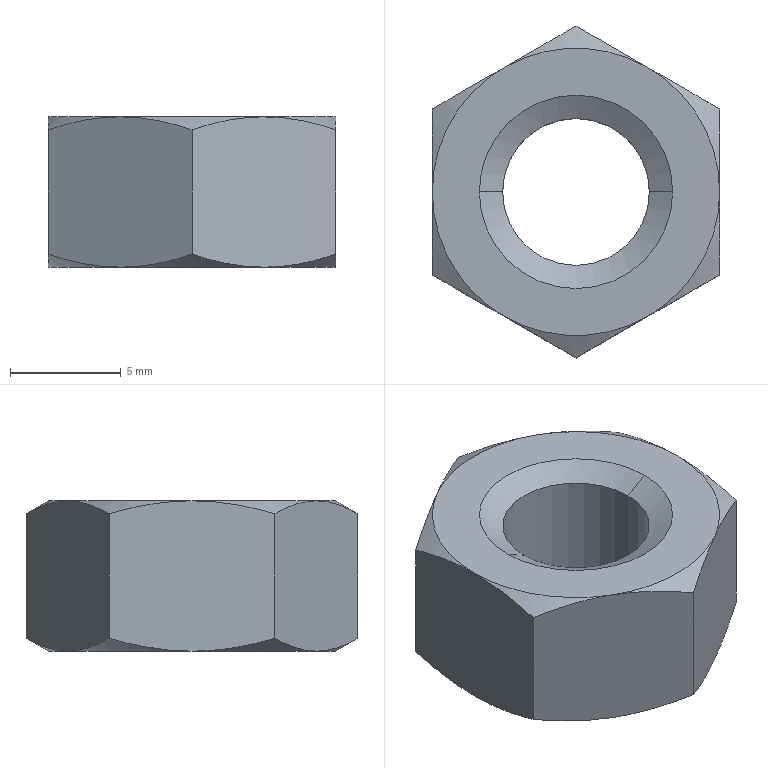Part | SolidWorks | features ICE 2, RevCut 2, Extrusion 1 | 1 solid | 26 faces | box 13 x 15.011 x 6.8 mm | volume 739.769 mm3 | cone 16 | plane 8 | cylinder 2 | commonest cylinder face diameters 6.647 x2
STEP:
#1=CARTESIAN_POINT('',(-3.323,0.,-6.193));
#2=VERTEX_POINT('',#1);
#3=CARTESIAN_POINT('',(3.323,0.,-6.193));
#4=VERTEX_POINT('',#3);
#5=CARTESIAN_POINT('',(0.,0.,-6.193));
#6=DIRECTION('',(0.,0.,1.));
#7=DIRECTION('',(1.,0.,0.));
#8=AXIS2_PLACEMENT_3D('',#5,#6,#7);
#9=CIRCLE('',#8,3.323);
#10=EDGE_CURVE('',#2,#4,#9,.T.);
#11=ORIENTED_EDGE('',*,*,#10,.T.);
#12=CARTESIAN_POINT('',(4.375,0.,-6.8));
#13=VERTEX_POINT('',#12);
#14=CARTESIAN_POINT('',(4.375,0.,-6.8));
#15=DIRECTION('',(0.866,0.,-0.5));
#16=VECTOR('',#15,1000.);
#17=LINE('',#14,#16);
#18=EDGE_CURVE('',#4,#13,#17,.T.);
#19=ORIENTED_EDGE('',*,*,#18,.T.);
#20=CARTESIAN_POINT('',(-4.375,0.,-6.8));
#21=VERTEX_POINT('',#20);
#22=CARTESIAN_POINT('',(0.,0.,-6.8));
#23=DIRECTION('',(0.,0.,1.));
#24=DIRECTION('',(1.,0.,0.));
#25=AXIS2_PLACEMENT_3D('',#22,#23,#24);
#26=CIRCLE('',#25,4.375);
#27=EDGE_CURVE('',#21,#13,#26,.T.);
#28=ORIENTED_EDGE('',*,*,#27,.F.);
#29=CARTESIAN_POINT('',(-4.375,0.,-6.8));
#30=DIRECTION('',(-0.866,0.,-0.5));
#31=VECTOR('',#30,1000.);
#32=LINE('',#29,#31);
#33=EDGE_CURVE('',#2,#21,#32,.T.);
#34=ORIENTED_EDGE('',*,*,#33,.F.);
#35=EDGE_LOOP('',(#11,#19,#28,#34));
#36=FACE_OUTER_BOUND('',#35,.T.);
#37=CARTESIAN_POINT('',(0.,0.,-6.8));
#38=DIRECTION('',(0.,0.,-1.));
#39=DIRECTION('',(-1.,0.,0.));
#40=AXIS2_PLACEMENT_3D('',#37,#38,#39);
#41=CONICAL_SURFACE('',#40,4.375,1.047);
#42=ADVANCED_FACE('',(#36),#41,.F.);
#43=CARTESIAN_POINT('',(-3.323,0.,-0.6071));
#44=VERTEX_POINT('',#43);
#45=CARTESIAN_POINT('',(3.323,0.,-0.6071));
#46=VERTEX_POINT('',#45);
#47=CARTESIAN_POINT('',(0.,0.,-0.6071));
#48=DIRECTION('',(0.,0.,1.));
#49=DIRECTION('',(1.,0.,0.));
#50=AXIS2_PLACEMENT_3D('',#47,#48,#49);
#51=CIRCLE('',#50,3.323);
#52=EDGE_CURVE('',#44,#46,#51,.T.);
#53=ORIENTED_EDGE('',*,*,#52,.F.);
#54=CARTESIAN_POINT('',(-4.375,0.,0.));
#55=VERTEX_POINT('',#54);
#56=CARTESIAN_POINT('',(-3.323,0.,-0.6071));
#57=DIRECTION('',(-0.866,0.,0.5));
#58=VECTOR('',#57,1000.);
#59=LINE('',#56,#58);
#60=EDGE_CURVE('',#44,#55,#59,.T.);
#61=ORIENTED_EDGE('',*,*,#60,.T.);
#62=CARTESIAN_POINT('',(4.375,0.,0.));
#63=VERTEX_POINT('',#62);
#64=CARTESIAN_POINT('',(0.,0.,0.));
#65=DIRECTION('',(0.,0.,1.));
#66=DIRECTION('',(1.,0.,0.));
#67=AXIS2_PLACEMENT_3D('',#64,#65,#66);
#68=CIRCLE('',#67,4.375);
#69=EDGE_CURVE('',#55,#63,#68,.T.);
#70=ORIENTED_EDGE('',*,*,#69,.T.);
#71=CARTESIAN_POINT('',(3.323,0.,-0.6071));
#72=DIRECTION('',(0.866,0.,0.5));
#73=VECTOR('',#72,1000.);
#74=LINE('',#71,#73);
#75=EDGE_CURVE('',#46,#63,#74,.T.);
#76=ORIENTED_EDGE('',*,*,#75,.F.);
#77=EDGE_LOOP('',(#53,#61,#70,#76));
#78=FACE_OUTER_BOUND('',#77,.T.);
#79=CARTESIAN_POINT('',(0.,0.,-0.6071));
#80=DIRECTION('',(0.,0.,1.));
#81=DIRECTION('',(1.,0.,0.));
#82=AXIS2_PLACEMENT_3D('',#79,#80,#81);
#83=CONICAL_SURFACE('',#82,3.323,1.047);
#84=ADVANCED_FACE('',(#78),#83,.F.);
#85=ORIENTED_EDGE('',*,*,#10,.F.);
#86=CARTESIAN_POINT('',(-3.323,0.,-6.8));
#87=DIRECTION('',(0.,0.,1.));
#88=VECTOR('',#87,1000.);
#89=LINE('',#86,#88);
#90=EDGE_CURVE('',#2,#44,#89,.T.);
#91=ORIENTED_EDGE('',*,*,#90,.T.);
#92=ORIENTED_EDGE('',*,*,#52,.T.);
#93=CARTESIAN_POINT('',(3.323,0.,-6.8));
#94=DIRECTION('',(0.,0.,1.));
#95=VECTOR('',#94,1000.);
#96=LINE('',#93,#95);
#97=EDGE_CURVE('',#4,#46,#96,.T.);
#98=ORIENTED_EDGE('',*,*,#97,.F.);
#99=EDGE_LOOP('',(#85,#91,#92,#98));
#100=FACE_OUTER_BOUND('',#99,.T.);
#101=CARTESIAN_POINT('',(0.,0.,-6.8));
#102=DIRECTION('',(0.,0.,1.));
#103=DIRECTION('',(1.,0.,0.));
#104=AXIS2_PLACEMENT_3D('',#101,#102,#103);
#105=CYLINDRICAL_SURFACE('',#104,3.323);
#106=ADVANCED_FACE('',(#100),#105,.F.);
#107=CARTESIAN_POINT('',(6.5,3.753,-6.219));
#108=VERTEX_POINT('',#107);
#109=CARTESIAN_POINT('',(6.5,3.753,-0.5806));
#110=VERTEX_POINT('',#109);
#111=CARTESIAN_POINT('',(6.5,3.753,-6.8));
#112=DIRECTION('',(0.,0.,1.));
#113=VECTOR('',#112,1000.);
#114=LINE('',#111,#113);
#115=EDGE_CURVE('',#108,#110,#114,.T.);
#116=ORIENTED_EDGE('',*,*,#115,.F.);
#117=CARTESIAN_POINT('',(3.25,5.629,-6.8));
#118=VERTEX_POINT('',#117);
#119=CARTESIAN_POINT('',(6.5,3.753,-6.219));
#120=CARTESIAN_POINT('',(5.968,4.06,-6.397));
#121=CARTESIAN_POINT('',(5.433,4.369,-6.543));
#122=CARTESIAN_POINT('',(4.351,4.994,-6.745));
#123=CARTESIAN_POINT('',(3.804,5.309,-6.8));
#124=CARTESIAN_POINT('',(3.25,5.629,-6.8));
#125=B_SPLINE_CURVE_WITH_KNOTS('',3,(#119,#120,#121,#122,#123,#124),.UNSPECIFIED.,.F.,.F.,(4,2,4),(0.000000238,0.001899,0.003797),.UNSPECIFIED.);
#126=EDGE_CURVE('',#108,#118,#125,.T.);
#127=ORIENTED_EDGE('',*,*,#126,.T.);
#128=CARTESIAN_POINT('',(0.,7.506,-6.219));
#129=VERTEX_POINT('',#128);
#130=CARTESIAN_POINT('',(3.25,5.629,-6.8));
#131=CARTESIAN_POINT('',(2.974,5.788,-6.8));
#132=CARTESIAN_POINT('',(2.697,5.948,-6.786));
#133=CARTESIAN_POINT('',(2.149,6.265,-6.733));
#134=CARTESIAN_POINT('',(1.877,6.422,-6.694));
#135=CARTESIAN_POINT('',(1.065,6.891,-6.542));
#136=CARTESIAN_POINT('',(0.5303,7.199,-6.396));
#137=CARTESIAN_POINT('',(0.,7.506,-6.219));
#138=B_SPLINE_CURVE_WITH_KNOTS('',3,(#130,#131,#132,#133,#134,#135,#136,#137),.UNSPECIFIED.,.F.,.F.,(4,2,2,4),(0.003797,0.004743,0.005689,0.00758),.UNSPECIFIED.);
#139=EDGE_CURVE('',#118,#129,#138,.T.);
#140=ORIENTED_EDGE('',*,*,#139,.T.);
#141=CARTESIAN_POINT('',(0.,7.506,-0.5806));
#142=VERTEX_POINT('',#141);
#143=CARTESIAN_POINT('',(0.,7.506,-6.8));
#144=DIRECTION('',(0.,0.,1.));
#145=VECTOR('',#144,1000.);
#146=LINE('',#143,#145);
#147=EDGE_CURVE('',#129,#142,#146,.T.);
#148=ORIENTED_EDGE('',*,*,#147,.T.);
#149=CARTESIAN_POINT('',(3.25,5.629,0.));
#150=VERTEX_POINT('',#149);
#151=CARTESIAN_POINT('',(0.,7.506,-0.5806));
#152=CARTESIAN_POINT('',(0.5317,7.199,-0.4033));
#153=CARTESIAN_POINT('',(1.067,6.889,-0.2573));
#154=CARTESIAN_POINT('',(2.149,6.265,-0.05533));
#155=CARTESIAN_POINT('',(2.696,5.949,0.));
#156=CARTESIAN_POINT('',(3.25,5.629,0.));
#157=B_SPLINE_CURVE_WITH_KNOTS('',3,(#151,#152,#153,#154,#155,#156),.UNSPECIFIED.,.F.,.F.,(4,2,4),(0.000000238,0.001899,0.003797),.UNSPECIFIED.);
#158=EDGE_CURVE('',#142,#150,#157,.T.);
#159=ORIENTED_EDGE('',*,*,#158,.T.);
#160=CARTESIAN_POINT('',(3.25,5.629,0.));
#161=CARTESIAN_POINT('',(3.526,5.47,0.));
#162=CARTESIAN_POINT('',(3.803,5.31,-0.01372));
#163=CARTESIAN_POINT('',(4.351,4.994,-0.06683));
#164=CARTESIAN_POINT('',(4.623,4.836,-0.1062));
#165=CARTESIAN_POINT('',(5.435,4.368,-0.2578));
#166=CARTESIAN_POINT('',(5.97,4.059,-0.4038));
#167=CARTESIAN_POINT('',(6.5,3.753,-0.5806));
#168=B_SPLINE_CURVE_WITH_KNOTS('',3,(#160,#161,#162,#163,#164,#165,#166,#167),.UNSPECIFIED.,.F.,.F.,(4,2,2,4),(0.003797,0.004743,0.005689,0.00758),.UNSPECIFIED.);
#169=EDGE_CURVE('',#150,#110,#168,.T.);
#170=ORIENTED_EDGE('',*,*,#169,.T.);
#171=EDGE_LOOP('',(#116,#127,#140,#148,#159,#170));
#172=FACE_OUTER_BOUND('',#171,.T.);
#173=CARTESIAN_POINT('',(6.5,3.753,-6.8));
#174=DIRECTION('',(0.5,0.866,0.));
#175=DIRECTION('',(-0.866,0.5,0.));
#176=AXIS2_PLACEMENT_3D('',#173,#174,#175);
#177=PLANE('',#176);
#178=ADVANCED_FACE('',(#172),#177,.T.);
#179=CARTESIAN_POINT('',(6.5,-3.753,-6.219));
#180=VERTEX_POINT('',#179);
#181=CARTESIAN_POINT('',(6.5,-3.753,-0.5806));
#182=VERTEX_POINT('',#181);
#183=CARTESIAN_POINT('',(6.5,-3.753,-6.8));
#184=DIRECTION('',(0.,0.,1.));
#185=VECTOR('',#184,1000.);
#186=LINE('',#183,#185);
#187=EDGE_CURVE('',#180,#182,#186,.T.);
#188=ORIENTED_EDGE('',*,*,#187,.F.);
#189=CARTESIAN_POINT('',(6.5,0.,-6.8));
#190=VERTEX_POINT('',#189);
#191=CARTESIAN_POINT('',(6.5,-3.753,-6.219));
#192=CARTESIAN_POINT('',(6.5,-3.142,-6.396));
#193=CARTESIAN_POINT('',(6.5,-2.517,-6.543));
#194=CARTESIAN_POINT('',(6.5,-1.264,-6.745));
#195=CARTESIAN_POINT('',(6.5,-0.6344,-6.8));
#196=CARTESIAN_POINT('',(6.5,0.,-6.8));
#197=B_SPLINE_CURVE_WITH_KNOTS('',3,(#191,#192,#193,#194,#195,#196),.UNSPECIFIED.,.F.,.F.,(4,2,4),(0.006797,0.008696,0.01059),.UNSPECIFIED.);
#198=EDGE_CURVE('',#180,#190,#197,.T.);
#199=ORIENTED_EDGE('',*,*,#198,.T.);
#200=CARTESIAN_POINT('',(6.5,0.,-6.8));
#201=CARTESIAN_POINT('',(6.5,0.6349,-6.8));
#202=CARTESIAN_POINT('',(6.5,1.278,-6.744));
#203=CARTESIAN_POINT('',(6.5,2.531,-6.54));
#204=CARTESIAN_POINT('',(6.5,3.146,-6.395));
#205=CARTESIAN_POINT('',(6.5,3.753,-6.219));
#206=B_SPLINE_CURVE_WITH_KNOTS('',3,(#200,#201,#202,#203,#204,#205),.UNSPECIFIED.,.F.,.F.,(4,2,4),(0.01059,0.01249,0.01439),.UNSPECIFIED.);
#207=EDGE_CURVE('',#190,#108,#206,.T.);
#208=ORIENTED_EDGE('',*,*,#207,.T.);
#209=ORIENTED_EDGE('',*,*,#115,.T.);
#210=CARTESIAN_POINT('',(6.5,0.,0.));
#211=VERTEX_POINT('',#210);
#212=CARTESIAN_POINT('',(6.5,3.753,-0.5806));
#213=CARTESIAN_POINT('',(6.5,3.146,-0.4054));
#214=CARTESIAN_POINT('',(6.5,2.531,-0.2595));
#215=CARTESIAN_POINT('',(6.5,1.278,-0.05609));
#216=CARTESIAN_POINT('',(6.5,0.6349,0.));
#217=CARTESIAN_POINT('',(6.5,0.,0.));
#218=B_SPLINE_CURVE_WITH_KNOTS('',3,(#212,#213,#214,#215,#216,#217),.UNSPECIFIED.,.F.,.F.,(4,2,4),(0.01671,0.01861,0.02052),.UNSPECIFIED.);
#219=EDGE_CURVE('',#110,#211,#218,.T.);
#220=ORIENTED_EDGE('',*,*,#219,.T.);
#221=CARTESIAN_POINT('',(6.5,0.,0.));
#222=CARTESIAN_POINT('',(6.5,-0.6344,0.));
#223=CARTESIAN_POINT('',(6.5,-1.264,-0.05455));
#224=CARTESIAN_POINT('',(6.5,-2.517,-0.2565));
#225=CARTESIAN_POINT('',(6.5,-3.142,-0.4043));
#226=CARTESIAN_POINT('',(6.5,-3.753,-0.5806));
#227=B_SPLINE_CURVE_WITH_KNOTS('',3,(#221,#222,#223,#224,#225,#226),.UNSPECIFIED.,.F.,.F.,(4,2,4),(0.02052,0.02242,0.02432),.UNSPECIFIED.);
#228=EDGE_CURVE('',#211,#182,#227,.T.);
#229=ORIENTED_EDGE('',*,*,#228,.T.);
#230=EDGE_LOOP('',(#188,#199,#208,#209,#220,#229));
#231=FACE_OUTER_BOUND('',#230,.T.);
#232=CARTESIAN_POINT('',(6.5,-3.753,-6.8));
#233=DIRECTION('',(1.,0.,0.));
#234=DIRECTION('',(0.,0.,-1.));
#235=AXIS2_PLACEMENT_3D('',#232,#233,#234);
#236=PLANE('',#235);
#237=ADVANCED_FACE('',(#231),#236,.T.);
#238=CARTESIAN_POINT('',(0.,-7.506,-6.219));
#239=VERTEX_POINT('',#238);
#240=CARTESIAN_POINT('',(0.,-7.506,-0.5806));
#241=VERTEX_POINT('',#240);
#242=CARTESIAN_POINT('',(0.,-7.506,-6.8));
#243=DIRECTION('',(0.,0.,1.));
#244=VECTOR('',#243,1000.);
#245=LINE('',#242,#244);
#246=EDGE_CURVE('',#239,#241,#245,.T.);
#247=ORIENTED_EDGE('',*,*,#246,.F.);
#248=CARTESIAN_POINT('',(3.25,-5.629,-6.8));
#249=VERTEX_POINT('',#248);
#250=CARTESIAN_POINT('',(0.,-7.506,-6.219));
#251=CARTESIAN_POINT('',(0.5317,-7.199,-6.397));
#252=CARTESIAN_POINT('',(1.067,-6.889,-6.543));
#253=CARTESIAN_POINT('',(2.149,-6.265,-6.745));
#254=CARTESIAN_POINT('',(2.696,-5.949,-6.8));
#255=CARTESIAN_POINT('',(3.25,-5.629,-6.8));
#256=B_SPLINE_CURVE_WITH_KNOTS('',3,(#250,#251,#252,#253,#254,#255),.UNSPECIFIED.,.F.,.F.,(4,2,4),(0.000000238,0.001899,0.003797),.UNSPECIFIED.);
#257=EDGE_CURVE('',#239,#249,#256,.T.);
#258=ORIENTED_EDGE('',*,*,#257,.T.);
#259=CARTESIAN_POINT('',(3.25,-5.629,-6.8));
#260=CARTESIAN_POINT('',(3.526,-5.47,-6.8));
#261=CARTESIAN_POINT('',(3.803,-5.31,-6.786));
#262=CARTESIAN_POINT('',(4.351,-4.994,-6.733));
#263=CARTESIAN_POINT('',(4.623,-4.836,-6.694));
#264=CARTESIAN_POINT('',(5.435,-4.368,-6.542));
#265=CARTESIAN_POINT('',(5.97,-4.059,-6.396));
#266=CARTESIAN_POINT('',(6.5,-3.753,-6.219));
#267=B_SPLINE_CURVE_WITH_KNOTS('',3,(#259,#260,#261,#262,#263,#264,#265,#266),.UNSPECIFIED.,.F.,.F.,(4,2,2,4),(0.003797,0.004743,0.005689,0.00758),.UNSPECIFIED.);
#268=EDGE_CURVE('',#249,#180,#267,.T.);
#269=ORIENTED_EDGE('',*,*,#268,.T.);
#270=ORIENTED_EDGE('',*,*,#187,.T.);
#271=CARTESIAN_POINT('',(3.25,-5.629,0.));
#272=VERTEX_POINT('',#271);
#273=CARTESIAN_POINT('',(6.5,-3.753,-0.5806));
#274=CARTESIAN_POINT('',(5.968,-4.06,-0.4033));
#275=CARTESIAN_POINT('',(5.433,-4.369,-0.2573));
#276=CARTESIAN_POINT('',(4.351,-4.994,-0.05533));
#277=CARTESIAN_POINT('',(3.804,-5.309,0.));
#278=CARTESIAN_POINT('',(3.25,-5.629,0.));
#279=B_SPLINE_CURVE_WITH_KNOTS('',3,(#273,#274,#275,#276,#277,#278),.UNSPECIFIED.,.F.,.F.,(4,2,4),(0.000000238,0.001899,0.003797),.UNSPECIFIED.);
#280=EDGE_CURVE('',#182,#272,#279,.T.);
#281=ORIENTED_EDGE('',*,*,#280,.T.);
#282=CARTESIAN_POINT('',(3.25,-5.629,0.));
#283=CARTESIAN_POINT('',(2.974,-5.788,0.));
#284=CARTESIAN_POINT('',(2.697,-5.948,-0.01372));
#285=CARTESIAN_POINT('',(2.149,-6.265,-0.06683));
#286=CARTESIAN_POINT('',(1.877,-6.422,-0.1062));
#287=CARTESIAN_POINT('',(1.065,-6.891,-0.2578));
#288=CARTESIAN_POINT('',(0.5303,-7.199,-0.4038));
#289=CARTESIAN_POINT('',(0.,-7.506,-0.5806));
#290=B_SPLINE_CURVE_WITH_KNOTS('',3,(#282,#283,#284,#285,#286,#287,#288,#289),.UNSPECIFIED.,.F.,.F.,(4,2,2,4),(0.003797,0.004743,0.005689,0.00758),.UNSPECIFIED.);
#291=EDGE_CURVE('',#272,#241,#290,.T.);
#292=ORIENTED_EDGE('',*,*,#291,.T.);
#293=EDGE_LOOP('',(#247,#258,#269,#270,#281,#292));
#294=FACE_OUTER_BOUND('',#293,.T.);
#295=CARTESIAN_POINT('',(0.,-7.506,-6.8));
#296=DIRECTION('',(0.5,-0.866,0.));
#297=DIRECTION('',(0.866,0.5,0.));
#298=AXIS2_PLACEMENT_3D('',#295,#296,#297);
#299=PLANE('',#298);
#300=ADVANCED_FACE('',(#294),#299,.T.);
#301=CARTESIAN_POINT('',(-6.5,-3.753,-6.219));
#302=VERTEX_POINT('',#301);
#303=CARTESIAN_POINT('',(-6.5,-3.753,-0.5806));
#304=VERTEX_POINT('',#303);
#305=CARTESIAN_POINT('',(-6.5,-3.753,-6.8));
#306=DIRECTION('',(0.,0.,1.));
#307=VECTOR('',#306,1000.);
#308=LINE('',#305,#307);
#309=EDGE_CURVE('',#302,#304,#308,.T.);
#310=ORIENTED_EDGE('',*,*,#309,.F.);
#311=CARTESIAN_POINT('',(-3.25,-5.629,-6.8));
#312=VERTEX_POINT('',#311);
#313=CARTESIAN_POINT('',(-6.5,-3.753,-6.219));
#314=CARTESIAN_POINT('',(-5.968,-4.06,-6.397));
#315=CARTESIAN_POINT('',(-5.433,-4.369,-6.543));
#316=CARTESIAN_POINT('',(-4.351,-4.994,-6.745));
#317=CARTESIAN_POINT('',(-3.804,-5.309,-6.8));
#318=CARTESIAN_POINT('',(-3.25,-5.629,-6.8));
#319=B_SPLINE_CURVE_WITH_KNOTS('',3,(#313,#314,#315,#316,#317,#318),.UNSPECIFIED.,.F.,.F.,(4,2,4),(0.000000238,0.001899,0.003797),.UNSPECIFIED.);
#320=EDGE_CURVE('',#302,#312,#319,.T.);
#321=ORIENTED_EDGE('',*,*,#320,.T.);
#322=CARTESIAN_POINT('',(-3.25,-5.629,-6.8));
#323=CARTESIAN_POINT('',(-2.974,-5.788,-6.8));
#324=CARTESIAN_POINT('',(-2.697,-5.948,-6.786));
#325=CARTESIAN_POINT('',(-2.149,-6.265,-6.733));
#326=CARTESIAN_POINT('',(-1.877,-6.422,-6.694));
#327=CARTESIAN_POINT('',(-1.065,-6.891,-6.542));
#328=CARTESIAN_POINT('',(-0.5303,-7.199,-6.396));
#329=CARTESIAN_POINT('',(0.,-7.506,-6.219));
#330=B_SPLINE_CURVE_WITH_KNOTS('',3,(#322,#323,#324,#325,#326,#327,#328,#329),.UNSPECIFIED.,.F.,.F.,(4,2,2,4),(0.003797,0.004743,0.005689,0.00758),.UNSPECIFIED.);
#331=EDGE_CURVE('',#312,#239,#330,.T.);
#332=ORIENTED_EDGE('',*,*,#331,.T.);
#333=ORIENTED_EDGE('',*,*,#246,.T.);
#334=CARTESIAN_POINT('',(-3.25,-5.629,0.));
#335=VERTEX_POINT('',#334);
#336=CARTESIAN_POINT('',(0.,-7.506,-0.5806));
#337=CARTESIAN_POINT('',(-0.5317,-7.199,-0.4033));
#338=CARTESIAN_POINT('',(-1.067,-6.889,-0.2573));
#339=CARTESIAN_POINT('',(-2.149,-6.265,-0.05533));
#340=CARTESIAN_POINT('',(-2.696,-5.949,0.));
#341=CARTESIAN_POINT('',(-3.25,-5.629,0.));
#342=B_SPLINE_CURVE_WITH_KNOTS('',3,(#336,#337,#338,#339,#340,#341),.UNSPECIFIED.,.F.,.F.,(4,2,4),(0.000000238,0.001899,0.003797),.UNSPECIFIED.);
#343=EDGE_CURVE('',#241,#335,#342,.T.);
#344=ORIENTED_EDGE('',*,*,#343,.T.);
#345=CARTESIAN_POINT('',(-3.25,-5.629,0.));
#346=CARTESIAN_POINT('',(-3.526,-5.47,0.));
#347=CARTESIAN_POINT('',(-3.803,-5.31,-0.01372));
#348=CARTESIAN_POINT('',(-4.351,-4.994,-0.06683));
#349=CARTESIAN_POINT('',(-4.623,-4.836,-0.1062));
#350=CARTESIAN_POINT('',(-5.435,-4.368,-0.2578));
#351=CARTESIAN_POINT('',(-5.97,-4.059,-0.4038));
#352=CARTESIAN_POINT('',(-6.5,-3.753,-0.5806));
#353=B_SPLINE_CURVE_WITH_KNOTS('',3,(#345,#346,#347,#348,#349,#350,#351,#352),.UNSPECIFIED.,.F.,.F.,(4,2,2,4),(0.003797,0.004743,0.005689,0.00758),.UNSPECIFIED.);
#354=EDGE_CURVE('',#335,#304,#353,.T.);
#355=ORIENTED_EDGE('',*,*,#354,.T.);
#356=EDGE_LOOP('',(#310,#321,#332,#333,#344,#355));
#357=FACE_OUTER_BOUND('',#356,.T.);
#358=CARTESIAN_POINT('',(-6.5,-3.753,-6.8));
#359=DIRECTION('',(-0.5,-0.866,0.));
#360=DIRECTION('',(0.866,-0.5,0.));
#361=AXIS2_PLACEMENT_3D('',#358,#359,#360);
#362=PLANE('',#361);
#363=ADVANCED_FACE('',(#357),#362,.T.);
#364=CARTESIAN_POINT('',(-6.5,3.753,-6.219));
#365=VERTEX_POINT('',#364);
#366=CARTESIAN_POINT('',(-6.5,3.753,-0.5806));
#367=VERTEX_POINT('',#366);
#368=CARTESIAN_POINT('',(-6.5,3.753,-6.8));
#369=DIRECTION('',(0.,0.,1.));
#370=VECTOR('',#369,1000.);
#371=LINE('',#368,#370);
#372=EDGE_CURVE('',#365,#367,#371,.T.);
#373=ORIENTED_EDGE('',*,*,#372,.F.);
#374=CARTESIAN_POINT('',(-6.5,0.,-6.8));
#375=VERTEX_POINT('',#374);
#376=CARTESIAN_POINT('',(-6.5,3.753,-6.219));
#377=CARTESIAN_POINT('',(-6.5,3.146,-6.395));
#378=CARTESIAN_POINT('',(-6.5,2.531,-6.54));
#379=CARTESIAN_POINT('',(-6.5,1.278,-6.744));
#380=CARTESIAN_POINT('',(-6.5,0.6349,-6.8));
#381=CARTESIAN_POINT('',(-6.5,0.,-6.8));
#382=B_SPLINE_CURVE_WITH_KNOTS('',3,(#376,#377,#378,#379,#380,#381),.UNSPECIFIED.,.F.,.F.,(4,2,4),(0.01671,0.01861,0.02052),.UNSPECIFIED.);
#383=EDGE_CURVE('',#365,#375,#382,.T.);
#384=ORIENTED_EDGE('',*,*,#383,.T.);
#385=CARTESIAN_POINT('',(-6.5,0.,-6.8));
#386=CARTESIAN_POINT('',(-6.5,-0.6344,-6.8));
#387=CARTESIAN_POINT('',(-6.5,-1.264,-6.745));
#388=CARTESIAN_POINT('',(-6.5,-2.517,-6.543));
#389=CARTESIAN_POINT('',(-6.5,-3.142,-6.396));
#390=CARTESIAN_POINT('',(-6.5,-3.753,-6.219));
#391=B_SPLINE_CURVE_WITH_KNOTS('',3,(#385,#386,#387,#388,#389,#390),.UNSPECIFIED.,.F.,.F.,(4,2,4),(0.02052,0.02242,0.02432),.UNSPECIFIED.);
#392=EDGE_CURVE('',#375,#302,#391,.T.);
#393=ORIENTED_EDGE('',*,*,#392,.T.);
#394=ORIENTED_EDGE('',*,*,#309,.T.);
#395=CARTESIAN_POINT('',(-6.5,0.,0.));
#396=VERTEX_POINT('',#395);
#397=CARTESIAN_POINT('',(-6.5,-3.753,-0.5806));
#398=CARTESIAN_POINT('',(-6.5,-3.142,-0.4043));
#399=CARTESIAN_POINT('',(-6.5,-2.517,-0.2565));
#400=CARTESIAN_POINT('',(-6.5,-1.264,-0.05455));
#401=CARTESIAN_POINT('',(-6.5,-0.6344,0.));
#402=CARTESIAN_POINT('',(-6.5,0.,0.));
#403=B_SPLINE_CURVE_WITH_KNOTS('',3,(#397,#398,#399,#400,#401,#402),.UNSPECIFIED.,.F.,.F.,(4,2,4),(0.006797,0.008696,0.01059),.UNSPECIFIED.);
#404=EDGE_CURVE('',#304,#396,#403,.T.);
#405=ORIENTED_EDGE('',*,*,#404,.T.);
#406=CARTESIAN_POINT('',(-6.5,0.,0.));
#407=CARTESIAN_POINT('',(-6.5,0.6349,0.));
#408=CARTESIAN_POINT('',(-6.5,1.278,-0.05609));
#409=CARTESIAN_POINT('',(-6.5,2.531,-0.2595));
#410=CARTESIAN_POINT('',(-6.5,3.146,-0.4054));
#411=CARTESIAN_POINT('',(-6.5,3.753,-0.5806));
#412=B_SPLINE_CURVE_WITH_KNOTS('',3,(#406,#407,#408,#409,#410,#411),.UNSPECIFIED.,.F.,.F.,(4,2,4),(0.01059,0.01249,0.01439),.UNSPECIFIED.);
#413=EDGE_CURVE('',#396,#367,#412,.T.);
#414=ORIENTED_EDGE('',*,*,#413,.T.);
#415=EDGE_LOOP('',(#373,#384,#393,#394,#405,#414));
#416=FACE_OUTER_BOUND('',#415,.T.);
#417=CARTESIAN_POINT('',(-6.5,3.753,-6.8));
#418=DIRECTION('',(-1.,0.,0.));
#419=DIRECTION('',(0.,0.,1.));
#420=AXIS2_PLACEMENT_3D('',#417,#418,#419);
#421=PLANE('',#420);
#422=ADVANCED_FACE('',(#416),#421,.T.);
#423=ORIENTED_EDGE('',*,*,#147,.F.);
#424=CARTESIAN_POINT('',(-3.25,5.629,-6.8));
#425=VERTEX_POINT('',#424);
#426=CARTESIAN_POINT('',(0.,7.506,-6.219));
#427=CARTESIAN_POINT('',(-0.5317,7.199,-6.397));
#428=CARTESIAN_POINT('',(-1.067,6.889,-6.543));
#429=CARTESIAN_POINT('',(-2.149,6.265,-6.745));
#430=CARTESIAN_POINT('',(-2.696,5.949,-6.8));
#431=CARTESIAN_POINT('',(-3.25,5.629,-6.8));
#432=B_SPLINE_CURVE_WITH_KNOTS('',3,(#426,#427,#428,#429,#430,#431),.UNSPECIFIED.,.F.,.F.,(4,2,4),(0.000000238,0.001899,0.003797),.UNSPECIFIED.);
#433=EDGE_CURVE('',#129,#425,#432,.T.);
#434=ORIENTED_EDGE('',*,*,#433,.T.);
#435=CARTESIAN_POINT('',(-3.25,5.629,-6.8));
#436=CARTESIAN_POINT('',(-3.526,5.47,-6.8));
#437=CARTESIAN_POINT('',(-3.803,5.31,-6.786));
#438=CARTESIAN_POINT('',(-4.351,4.994,-6.733));
#439=CARTESIAN_POINT('',(-4.623,4.836,-6.694));
#440=CARTESIAN_POINT('',(-5.435,4.368,-6.542));
#441=CARTESIAN_POINT('',(-5.97,4.059,-6.396));
#442=CARTESIAN_POINT('',(-6.5,3.753,-6.219));
#443=B_SPLINE_CURVE_WITH_KNOTS('',3,(#435,#436,#437,#438,#439,#440,#441,#442),.UNSPECIFIED.,.F.,.F.,(4,2,2,4),(0.003797,0.004743,0.005689,0.00758),.UNSPECIFIED.);
#444=EDGE_CURVE('',#425,#365,#443,.T.);
#445=ORIENTED_EDGE('',*,*,#444,.T.);
#446=ORIENTED_EDGE('',*,*,#372,.T.);
#447=CARTESIAN_POINT('',(-3.25,5.629,0.));
#448=VERTEX_POINT('',#447);
#449=CARTESIAN_POINT('',(-6.5,3.753,-0.5806));
#450=CARTESIAN_POINT('',(-5.968,4.06,-0.4033));
#451=CARTESIAN_POINT('',(-5.433,4.369,-0.2573));
#452=CARTESIAN_POINT('',(-4.351,4.994,-0.05533));
#453=CARTESIAN_POINT('',(-3.804,5.309,0.));
#454=CARTESIAN_POINT('',(-3.25,5.629,0.));
#455=B_SPLINE_CURVE_WITH_KNOTS('',3,(#449,#450,#451,#452,#453,#454),.UNSPECIFIED.,.F.,.F.,(4,2,4),(0.000000238,0.001899,0.003797),.UNSPECIFIED.);
#456=EDGE_CURVE('',#367,#448,#455,.T.);
#457=ORIENTED_EDGE('',*,*,#456,.T.);
#458=CARTESIAN_POINT('',(-3.25,5.629,0.));
#459=CARTESIAN_POINT('',(-2.974,5.788,0.));
#460=CARTESIAN_POINT('',(-2.697,5.948,-0.01372));
#461=CARTESIAN_POINT('',(-2.149,6.265,-0.06683));
#462=CARTESIAN_POINT('',(-1.877,6.422,-0.1062));
#463=CARTESIAN_POINT('',(-1.065,6.891,-0.2578));
#464=CARTESIAN_POINT('',(-0.5303,7.199,-0.4038));
#465=CARTESIAN_POINT('',(0.,7.506,-0.5806));
#466=B_SPLINE_CURVE_WITH_KNOTS('',3,(#458,#459,#460,#461,#462,#463,#464,#465),.UNSPECIFIED.,.F.,.F.,(4,2,2,4),(0.003797,0.004743,0.005689,0.00758),.UNSPECIFIED.);
#467=EDGE_CURVE('',#448,#142,#466,.T.);
#468=ORIENTED_EDGE('',*,*,#467,.T.);
#469=EDGE_LOOP('',(#423,#434,#445,#446,#457,#468));
#470=FACE_OUTER_BOUND('',#469,.T.);
#471=CARTESIAN_POINT('',(0.,7.506,-6.8));
#472=DIRECTION('',(-0.5,0.866,0.));
#473=DIRECTION('',(-0.866,-0.5,0.));
#474=AXIS2_PLACEMENT_3D('',#471,#472,#473);
#475=PLANE('',#474);
#476=ADVANCED_FACE('',(#470),#475,.T.);
#477=ORIENTED_EDGE('',*,*,#27,.T.);
#478=CARTESIAN_POINT('',(0.,0.,-6.8));
#479=DIRECTION('',(0.,0.,1.));
#480=DIRECTION('',(1.,0.,0.));
#481=AXIS2_PLACEMENT_3D('',#478,#479,#480);
#482=CIRCLE('',#481,4.375);
#483=EDGE_CURVE('',#13,#21,#482,.T.);
#484=ORIENTED_EDGE('',*,*,#483,.T.);
#485=EDGE_LOOP('',(#477,#484));
#486=FACE_BOUND('',#485,.T.);
#487=CARTESIAN_POINT('',(0.,0.,-6.8));
#488=DIRECTION('',(0.,0.,1.));
#489=DIRECTION('',(1.,0.,0.));
#490=AXIS2_PLACEMENT_3D('',#487,#488,#489);
#491=CIRCLE('',#490,6.5);
#492=EDGE_CURVE('',#190,#118,#491,.T.);
#493=ORIENTED_EDGE('',*,*,#492,.F.);
#494=CARTESIAN_POINT('',(0.,0.,-6.8));
#495=DIRECTION('',(0.,0.,1.));
#496=DIRECTION('',(1.,0.,0.));
#497=AXIS2_PLACEMENT_3D('',#494,#495,#496);
#498=CIRCLE('',#497,6.5);
#499=EDGE_CURVE('',#249,#190,#498,.T.);
#500=ORIENTED_EDGE('',*,*,#499,.F.);
#501=CARTESIAN_POINT('',(0.,0.,-6.8));
#502=DIRECTION('',(0.,0.,1.));
#503=DIRECTION('',(1.,0.,0.));
#504=AXIS2_PLACEMENT_3D('',#501,#502,#503);
#505=CIRCLE('',#504,6.5);
#506=EDGE_CURVE('',#312,#249,#505,.T.);
#507=ORIENTED_EDGE('',*,*,#506,.F.);
#508=CARTESIAN_POINT('',(0.,0.,-6.8));
#509=DIRECTION('',(0.,0.,1.));
#510=DIRECTION('',(1.,0.,0.));
#511=AXIS2_PLACEMENT_3D('',#508,#509,#510);
#512=CIRCLE('',#511,6.5);
#513=EDGE_CURVE('',#375,#312,#512,.T.);
#514=ORIENTED_EDGE('',*,*,#513,.F.);
#515=CARTESIAN_POINT('',(0.,0.,-6.8));
#516=DIRECTION('',(0.,0.,-1.));
#517=DIRECTION('',(-1.,0.,0.));
#518=AXIS2_PLACEMENT_3D('',#515,#516,#517);
#519=CIRCLE('',#518,6.5);
#520=EDGE_CURVE('',#375,#425,#519,.T.);
#521=ORIENTED_EDGE('',*,*,#520,.T.);
#522=CARTESIAN_POINT('',(0.,0.,-6.8));
#523=DIRECTION('',(0.,0.,1.));
#524=DIRECTION('',(1.,0.,0.));
#525=AXIS2_PLACEMENT_3D('',#522,#523,#524);
#526=CIRCLE('',#525,6.5);
#527=EDGE_CURVE('',#118,#425,#526,.T.);
#528=ORIENTED_EDGE('',*,*,#527,.F.);
#529=EDGE_LOOP('',(#493,#500,#507,#514,#521,#528));
#530=FACE_OUTER_BOUND('',#529,.T.);
#531=CARTESIAN_POINT('',(0.,7.506,-6.8));
#532=DIRECTION('',(0.,0.,1.));
#533=DIRECTION('',(1.,0.,0.));
#534=AXIS2_PLACEMENT_3D('',#531,#532,#533);
#535=PLANE('',#534);
#536=ADVANCED_FACE('',(#486,#530),#535,.F.);
#537=CARTESIAN_POINT('',(0.,0.,0.));
#538=DIRECTION('',(0.,0.,1.));
#539=DIRECTION('',(1.,0.,0.));
#540=AXIS2_PLACEMENT_3D('',#537,#538,#539);
#541=CIRCLE('',#540,4.375);
#542=EDGE_CURVE('',#63,#55,#541,.T.);
#543=ORIENTED_EDGE('',*,*,#542,.F.);
#544=ORIENTED_EDGE('',*,*,#69,.F.);
#545=EDGE_LOOP('',(#543,#544));
#546=FACE_BOUND('',#545,.T.);
#547=CARTESIAN_POINT('',(0.,0.,0.));
#548=DIRECTION('',(0.,0.,1.));
#549=DIRECTION('',(1.,0.,0.));
#550=AXIS2_PLACEMENT_3D('',#547,#548,#549);
#551=CIRCLE('',#550,6.5);
#552=EDGE_CURVE('',#272,#211,#551,.T.);
#553=ORIENTED_EDGE('',*,*,#552,.T.);
#554=CARTESIAN_POINT('',(0.,0.,0.));
#555=DIRECTION('',(0.,0.,1.));
#556=DIRECTION('',(1.,0.,0.));
#557=AXIS2_PLACEMENT_3D('',#554,#555,#556);
#558=CIRCLE('',#557,6.5);
#559=EDGE_CURVE('',#211,#150,#558,.T.);
#560=ORIENTED_EDGE('',*,*,#559,.T.);
#561=CARTESIAN_POINT('',(0.,0.,0.));
#562=DIRECTION('',(0.,0.,1.));
#563=DIRECTION('',(1.,0.,0.));
#564=AXIS2_PLACEMENT_3D('',#561,#562,#563);
#565=CIRCLE('',#564,6.5);
#566=EDGE_CURVE('',#150,#448,#565,.T.);
#567=ORIENTED_EDGE('',*,*,#566,.T.);
#568=CARTESIAN_POINT('',(0.,0.,0.));
#569=DIRECTION('',(0.,0.,1.));
#570=DIRECTION('',(1.,0.,0.));
#571=AXIS2_PLACEMENT_3D('',#568,#569,#570);
#572=CIRCLE('',#571,6.5);
#573=EDGE_CURVE('',#448,#396,#572,.T.);
#574=ORIENTED_EDGE('',*,*,#573,.T.);
#575=CARTESIAN_POINT('',(0.,0.,0.));
#576=DIRECTION('',(0.,0.,1.));
#577=DIRECTION('',(1.,0.,0.));
#578=AXIS2_PLACEMENT_3D('',#575,#576,#577);
#579=CIRCLE('',#578,6.5);
#580=EDGE_CURVE('',#396,#335,#579,.T.);
#581=ORIENTED_EDGE('',*,*,#580,.T.);
#582=CARTESIAN_POINT('',(0.,0.,0.));
#583=DIRECTION('',(0.,0.,1.));
#584=DIRECTION('',(1.,0.,0.));
#585=AXIS2_PLACEMENT_3D('',#582,#583,#584);
#586=CIRCLE('',#585,6.5);
#587=EDGE_CURVE('',#335,#272,#586,.T.);
#588=ORIENTED_EDGE('',*,*,#587,.T.);
#589=EDGE_LOOP('',(#553,#560,#567,#574,#581,#588));
#590=FACE_OUTER_BOUND('',#589,.T.);
#591=CARTESIAN_POINT('',(0.,7.506,0.));
#592=DIRECTION('',(0.,0.,1.));
#593=DIRECTION('',(1.,0.,0.));
#594=AXIS2_PLACEMENT_3D('',#591,#592,#593);
#595=PLANE('',#594);
#596=ADVANCED_FACE('',(#546,#590),#595,.T.);
#597=ORIENTED_EDGE('',*,*,#90,.F.);
#598=CARTESIAN_POINT('',(0.,0.,-6.193));
#599=DIRECTION('',(0.,0.,1.));
#600=DIRECTION('',(1.,0.,0.));
#601=AXIS2_PLACEMENT_3D('',#598,#599,#600);
#602=CIRCLE('',#601,3.323);
#603=EDGE_CURVE('',#4,#2,#602,.T.);
#604=ORIENTED_EDGE('',*,*,#603,.F.);
#605=ORIENTED_EDGE('',*,*,#97,.T.);
#606=CARTESIAN_POINT('',(0.,0.,-0.6071));
#607=DIRECTION('',(0.,0.,1.));
#608=DIRECTION('',(1.,0.,0.));
#609=AXIS2_PLACEMENT_3D('',#606,#607,#608);
#610=CIRCLE('',#609,3.323);
#611=EDGE_CURVE('',#46,#44,#610,.T.);
#612=ORIENTED_EDGE('',*,*,#611,.T.);
#613=EDGE_LOOP('',(#597,#604,#605,#612));
#614=FACE_OUTER_BOUND('',#613,.T.);
#615=CARTESIAN_POINT('',(0.,0.,-6.8));
#616=DIRECTION('',(0.,0.,1.));
#617=DIRECTION('',(1.,0.,0.));
#618=AXIS2_PLACEMENT_3D('',#615,#616,#617);
#619=CYLINDRICAL_SURFACE('',#618,3.323);
#620=ADVANCED_FACE('',(#614),#619,.F.);
#621=ORIENTED_EDGE('',*,*,#60,.F.);
#622=ORIENTED_EDGE('',*,*,#611,.F.);
#623=ORIENTED_EDGE('',*,*,#75,.T.);
#624=ORIENTED_EDGE('',*,*,#542,.T.);
#625=EDGE_LOOP('',(#621,#622,#623,#624));
#626=FACE_OUTER_BOUND('',#625,.T.);
#627=CARTESIAN_POINT('',(0.,0.,-0.6071));
#628=DIRECTION('',(0.,0.,1.));
#629=DIRECTION('',(1.,0.,0.));
#630=AXIS2_PLACEMENT_3D('',#627,#628,#629);
#631=CONICAL_SURFACE('',#630,3.323,1.047);
#632=ADVANCED_FACE('',(#626),#631,.F.);
#633=ORIENTED_EDGE('',*,*,#18,.F.);
#634=ORIENTED_EDGE('',*,*,#603,.T.);
#635=ORIENTED_EDGE('',*,*,#33,.T.);
#636=ORIENTED_EDGE('',*,*,#483,.F.);
#637=EDGE_LOOP('',(#633,#634,#635,#636));
#638=FACE_OUTER_BOUND('',#637,.T.);
#639=CARTESIAN_POINT('',(0.,0.,-6.8));
#640=DIRECTION('',(0.,0.,-1.));
#641=DIRECTION('',(-1.,0.,0.));
#642=AXIS2_PLACEMENT_3D('',#639,#640,#641);
#643=CONICAL_SURFACE('',#642,4.375,1.047);
#644=ADVANCED_FACE('',(#638),#643,.F.);
#645=ORIENTED_EDGE('',*,*,#467,.F.);
#646=ORIENTED_EDGE('',*,*,#566,.F.);
#647=ORIENTED_EDGE('',*,*,#158,.F.);
#648=EDGE_LOOP('',(#645,#646,#647));
#649=FACE_OUTER_BOUND('',#648,.T.);
#650=CARTESIAN_POINT('',(0.,0.,0.));
#651=DIRECTION('',(0.,0.,-1.));
#652=DIRECTION('',(1.,0.,0.));
#653=AXIS2_PLACEMENT_3D('',#650,#651,#652);
#654=CONICAL_SURFACE('',#653,6.5,1.047);
#655=ADVANCED_FACE('',(#649),#654,.T.);
#656=ORIENTED_EDGE('',*,*,#573,.F.);
#657=ORIENTED_EDGE('',*,*,#456,.F.);
#658=ORIENTED_EDGE('',*,*,#413,.F.);
#659=EDGE_LOOP('',(#656,#657,#658));
#660=FACE_OUTER_BOUND('',#659,.T.);
#661=CARTESIAN_POINT('',(0.,0.,0.));
#662=DIRECTION('',(0.,0.,-1.));
#663=DIRECTION('',(1.,0.,0.));
#664=AXIS2_PLACEMENT_3D('',#661,#662,#663);
#665=CONICAL_SURFACE('',#664,6.5,1.047);
#666=ADVANCED_FACE('',(#660),#665,.T.);
#667=ORIENTED_EDGE('',*,*,#580,.F.);
#668=ORIENTED_EDGE('',*,*,#404,.F.);
#669=ORIENTED_EDGE('',*,*,#354,.F.);
#670=EDGE_LOOP('',(#667,#668,#669));
#671=FACE_OUTER_BOUND('',#670,.T.);
#672=CARTESIAN_POINT('',(0.,0.,0.));
#673=DIRECTION('',(0.,0.,-1.));
#674=DIRECTION('',(1.,0.,0.));
#675=AXIS2_PLACEMENT_3D('',#672,#673,#674);
#676=CONICAL_SURFACE('',#675,6.5,1.047);
#677=ADVANCED_FACE('',(#671),#676,.T.);
#678=ORIENTED_EDGE('',*,*,#587,.F.);
#679=ORIENTED_EDGE('',*,*,#343,.F.);
#680=ORIENTED_EDGE('',*,*,#291,.F.);
#681=EDGE_LOOP('',(#678,#679,#680));
#682=FACE_OUTER_BOUND('',#681,.T.);
#683=CARTESIAN_POINT('',(0.,0.,0.));
#684=DIRECTION('',(0.,0.,-1.));
#685=DIRECTION('',(1.,0.,0.));
#686=AXIS2_PLACEMENT_3D('',#683,#684,#685);
#687=CONICAL_SURFACE('',#686,6.5,1.047);
#688=ADVANCED_FACE('',(#682),#687,.T.);
#689=ORIENTED_EDGE('',*,*,#552,.F.);
#690=ORIENTED_EDGE('',*,*,#280,.F.);
#691=ORIENTED_EDGE('',*,*,#228,.F.);
#692=EDGE_LOOP('',(#689,#690,#691));
#693=FACE_OUTER_BOUND('',#692,.T.);
#694=CARTESIAN_POINT('',(0.,0.,0.));
#695=DIRECTION('',(0.,0.,-1.));
#696=DIRECTION('',(1.,0.,0.));
#697=AXIS2_PLACEMENT_3D('',#694,#695,#696);
#698=CONICAL_SURFACE('',#697,6.5,1.047);
#699=ADVANCED_FACE('',(#693),#698,.T.);
#700=ORIENTED_EDGE('',*,*,#559,.F.);
#701=ORIENTED_EDGE('',*,*,#219,.F.);
#702=ORIENTED_EDGE('',*,*,#169,.F.);
#703=EDGE_LOOP('',(#700,#701,#702));
#704=FACE_OUTER_BOUND('',#703,.T.);
#705=CARTESIAN_POINT('',(0.,0.,0.));
#706=DIRECTION('',(0.,0.,-1.));
#707=DIRECTION('',(1.,0.,0.));
#708=AXIS2_PLACEMENT_3D('',#705,#706,#707);
#709=CONICAL_SURFACE('',#708,6.5,1.047);
#710=ADVANCED_FACE('',(#704),#709,.T.);
#711=ORIENTED_EDGE('',*,*,#499,.T.);
#712=ORIENTED_EDGE('',*,*,#198,.F.);
#713=ORIENTED_EDGE('',*,*,#268,.F.);
#714=EDGE_LOOP('',(#711,#712,#713));
#715=FACE_OUTER_BOUND('',#714,.T.);
#716=CARTESIAN_POINT('',(0.,0.,-6.8));
#717=DIRECTION('',(0.,0.,1.));
#718=DIRECTION('',(-1.,0.,0.));
#719=AXIS2_PLACEMENT_3D('',#716,#717,#718);
#720=CONICAL_SURFACE('',#719,6.5,1.047);
#721=ADVANCED_FACE('',(#715),#720,.T.);
#722=ORIENTED_EDGE('',*,*,#331,.F.);
#723=ORIENTED_EDGE('',*,*,#506,.T.);
#724=ORIENTED_EDGE('',*,*,#257,.F.);
#725=EDGE_LOOP('',(#722,#723,#724));
#726=FACE_OUTER_BOUND('',#725,.T.);
#727=CARTESIAN_POINT('',(0.,0.,-6.8));
#728=DIRECTION('',(0.,0.,1.));
#729=DIRECTION('',(-1.,0.,0.));
#730=AXIS2_PLACEMENT_3D('',#727,#728,#729);
#731=CONICAL_SURFACE('',#730,6.5,1.047);
#732=ADVANCED_FACE('',(#726),#731,.T.);
#733=ORIENTED_EDGE('',*,*,#392,.F.);
#734=ORIENTED_EDGE('',*,*,#513,.T.);
#735=ORIENTED_EDGE('',*,*,#320,.F.);
#736=EDGE_LOOP('',(#733,#734,#735));
#737=FACE_OUTER_BOUND('',#736,.T.);
#738=CARTESIAN_POINT('',(0.,0.,-6.8));
#739=DIRECTION('',(0.,0.,1.));
#740=DIRECTION('',(-1.,0.,0.));
#741=AXIS2_PLACEMENT_3D('',#738,#739,#740);
#742=CONICAL_SURFACE('',#741,6.5,1.047);
#743=ADVANCED_FACE('',(#737),#742,.T.);
#744=ORIENTED_EDGE('',*,*,#444,.F.);
#745=ORIENTED_EDGE('',*,*,#520,.F.);
#746=ORIENTED_EDGE('',*,*,#383,.F.);
#747=EDGE_LOOP('',(#744,#745,#746));
#748=FACE_OUTER_BOUND('',#747,.T.);
#749=CARTESIAN_POINT('',(0.,0.,-6.8));
#750=DIRECTION('',(0.,0.,1.));
#751=DIRECTION('',(-1.,0.,0.));
#752=AXIS2_PLACEMENT_3D('',#749,#750,#751);
#753=CONICAL_SURFACE('',#752,6.5,1.047);
#754=ADVANCED_FACE('',(#748),#753,.T.);
#755=ORIENTED_EDGE('',*,*,#527,.T.);
#756=ORIENTED_EDGE('',*,*,#433,.F.);
#757=ORIENTED_EDGE('',*,*,#139,.F.);
#758=EDGE_LOOP('',(#755,#756,#757));
#759=FACE_OUTER_BOUND('',#758,.T.);
#760=CARTESIAN_POINT('',(0.,0.,-6.8));
#761=DIRECTION('',(0.,0.,1.));
#762=DIRECTION('',(-1.,0.,0.));
#763=AXIS2_PLACEMENT_3D('',#760,#761,#762);
#764=CONICAL_SURFACE('',#763,6.5,1.047);
#765=ADVANCED_FACE('',(#759),#764,.T.);
#766=ORIENTED_EDGE('',*,*,#492,.T.);
#767=ORIENTED_EDGE('',*,*,#126,.F.);
#768=ORIENTED_EDGE('',*,*,#207,.F.);
#769=EDGE_LOOP('',(#766,#767,#768));
#770=FACE_OUTER_BOUND('',#769,.T.);
#771=CARTESIAN_POINT('',(0.,0.,-6.8));
#772=DIRECTION('',(0.,0.,1.));
#773=DIRECTION('',(-1.,0.,0.));
#774=AXIS2_PLACEMENT_3D('',#771,#772,#773);
#775=CONICAL_SURFACE('',#774,6.5,1.047);
#776=ADVANCED_FACE('',(#770),#775,.T.);
#777=CLOSED_SHELL('',(#42,#84,#106,#178,#237,#300,#363,#422,#476,#536,#596,#620,#632,#644,#655,#666,#677,#688,#699,#710,#721,#732,#743,#754,#765,#776));
#778=MANIFOLD_SOLID_BREP('',#777);
#779=CARTESIAN_POINT('',(0.,0.,0.));
#780=DIRECTION('',(0.,0.,1.));
#781=DIRECTION('',(1.,0.,0.));
#782=AXIS2_PLACEMENT_3D('',#779,#780,#781);
#783=(LENGTH_UNIT()NAMED_UNIT(*)SI_UNIT(.MILLI.,.METRE.));
#784=UNCERTAINTY_MEASURE_WITH_UNIT(LENGTH_MEASURE(0.00001),#783,'','');
#785=(NAMED_UNIT(*)PLANE_ANGLE_UNIT()SI_UNIT($,.RADIAN.));
#786=(NAMED_UNIT(*)SI_UNIT($,.STERADIAN.)SOLID_ANGLE_UNIT());
#787=(GEOMETRIC_REPRESENTATION_CONTEXT(3)GLOBAL_UNCERTAINTY_ASSIGNED_CONTEXT((#784))GLOBAL_UNIT_ASSIGNED_CONTEXT((#783,#785,#786))REPRESENTATION_CONTEXT('',''));
#788=ADVANCED_BREP_SHAPE_REPRESENTATION('',(#778,#782),#787);